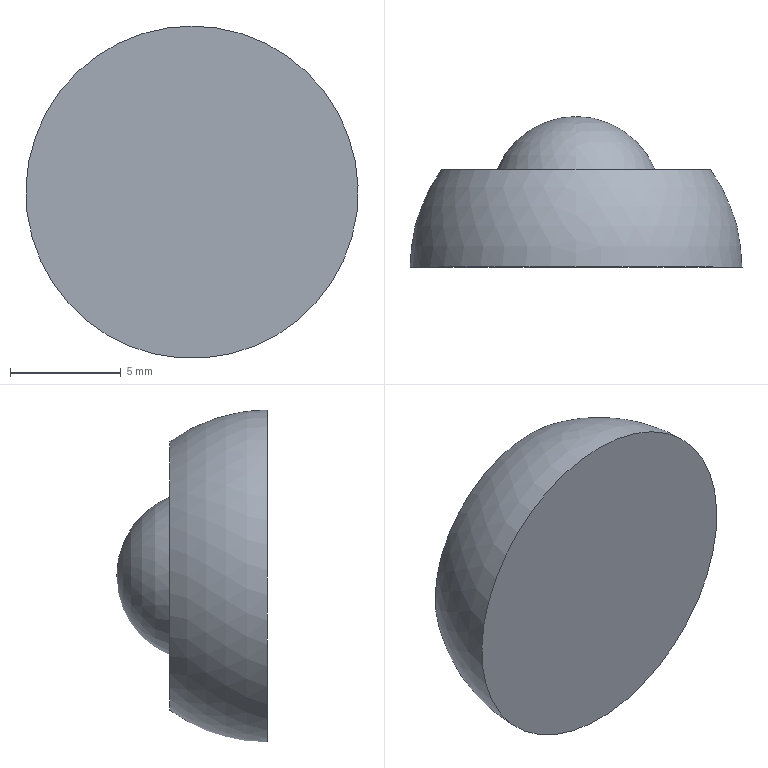Part | NX | features MFD10-WL40_1 2 | 1 solid | 4 faces | box 15 x 6.8 x 15 mm | volume 743.606 mm3 | plane 2 | sphere 2
STEP:
#1=CARTESIAN_POINT('',(275.029,-463.352,93.8));
#2=VERTEX_POINT('',#1);
#3=CARTESIAN_POINT('',(275.029,-463.352,87.725));
#4=DIRECTION('',(0.,-1.,0.));
#5=DIRECTION('',(0.,0.,1.));
#6=AXIS2_PLACEMENT_3D('',#3,#4,#5);
#7=CIRCLE('',#6,6.075);
#8=EDGE_CURVE('',#2,#2,#7,.T.);
#9=ORIENTED_EDGE('',*,*,#8,.F.);
#10=EDGE_LOOP('',(#9));
#11=FACE_BOUND('',#10,.T.);
#12=CARTESIAN_POINT('',(275.029,-463.352,91.3));
#13=VERTEX_POINT('',#12);
#14=CARTESIAN_POINT('',(275.029,-463.352,87.725));
#15=DIRECTION('',(0.,-1.,0.));
#16=DIRECTION('',(0.,0.,1.));
#17=AXIS2_PLACEMENT_3D('',#14,#15,#16);
#18=CIRCLE('',#17,3.575);
#19=EDGE_CURVE('',#13,#13,#18,.T.);
#20=ORIENTED_EDGE('',*,*,#19,.T.);
#21=EDGE_LOOP('',(#20));
#22=FACE_BOUND('',#21,.T.);
#23=CARTESIAN_POINT('',(275.029,-463.352,93.8));
#24=DIRECTION('',(0.,1.,0.));
#25=DIRECTION('',(-1.,0.,0.));
#26=AXIS2_PLACEMENT_3D('',#23,#24,#25);
#27=PLANE('',#26);
#28=ADVANCED_FACE('',(#11,#22),#27,.T.);
#29=ORIENTED_EDGE('',*,*,#19,.F.);
#30=EDGE_LOOP('',(#29));
#31=FACE_BOUND('',#30,.T.);
#32=CARTESIAN_POINT('',(275.029,-464.812,87.725));
#33=DIRECTION('',(0.,-1.,0.));
#34=DIRECTION('',(0.,0.,1.));
#35=AXIS2_PLACEMENT_3D('',#32,#33,#34);
#36=SPHERICAL_SURFACE('',#35,3.862);
#37=ADVANCED_FACE('',(#31),#36,.T.);
#38=CARTESIAN_POINT('',(275.029,-467.75,95.225));
#39=VERTEX_POINT('',#38);
#40=CARTESIAN_POINT('',(275.029,-467.75,87.725));
#41=DIRECTION('',(0.,-1.,0.));
#42=DIRECTION('',(0.,0.,1.));
#43=AXIS2_PLACEMENT_3D('',#40,#41,#42);
#44=CIRCLE('',#43,7.5);
#45=EDGE_CURVE('',#39,#39,#44,.T.);
#46=ORIENTED_EDGE('',*,*,#45,.T.);
#47=EDGE_LOOP('',(#46));
#48=FACE_BOUND('',#47,.T.);
#49=CARTESIAN_POINT('',(275.029,-467.75,87.725));
#50=DIRECTION('',(0.,-1.,0.));
#51=DIRECTION('',(0.,0.,1.));
#52=AXIS2_PLACEMENT_3D('',#49,#50,#51);
#53=PLANE('',#52);
#54=ADVANCED_FACE('',(#48),#53,.T.);
#55=ORIENTED_EDGE('',*,*,#8,.T.);
#56=EDGE_LOOP('',(#55));
#57=FACE_BOUND('',#56,.T.);
#58=ORIENTED_EDGE('',*,*,#45,.F.);
#59=EDGE_LOOP('',(#58));
#60=FACE_BOUND('',#59,.T.);
#61=CARTESIAN_POINT('',(275.029,-467.75,87.725));
#62=DIRECTION('',(0.,-1.,0.));
#63=DIRECTION('',(0.,0.,1.));
#64=AXIS2_PLACEMENT_3D('',#61,#62,#63);
#65=SPHERICAL_SURFACE('',#64,7.5);
#66=ADVANCED_FACE('',(#57,#60),#65,.T.);
#67=CLOSED_SHELL('',(#28,#37,#54,#66));
#68=MANIFOLD_SOLID_BREP('',#67);
#69=(LENGTH_UNIT()NAMED_UNIT(*)SI_UNIT(.MILLI.,.METRE.));
#70=UNCERTAINTY_MEASURE_WITH_UNIT(LENGTH_MEASURE(0.00001),#69,'','');
#71=(NAMED_UNIT(*)PLANE_ANGLE_UNIT()SI_UNIT($,.RADIAN.));
#72=(NAMED_UNIT(*)SI_UNIT($,.STERADIAN.)SOLID_ANGLE_UNIT());
#73=(GEOMETRIC_REPRESENTATION_CONTEXT(3)GLOBAL_UNCERTAINTY_ASSIGNED_CONTEXT((#70))GLOBAL_UNIT_ASSIGNED_CONTEXT((#69,#71,#72))REPRESENTATION_CONTEXT('',''));
#74=ADVANCED_BREP_SHAPE_REPRESENTATION('',(#68),#73);